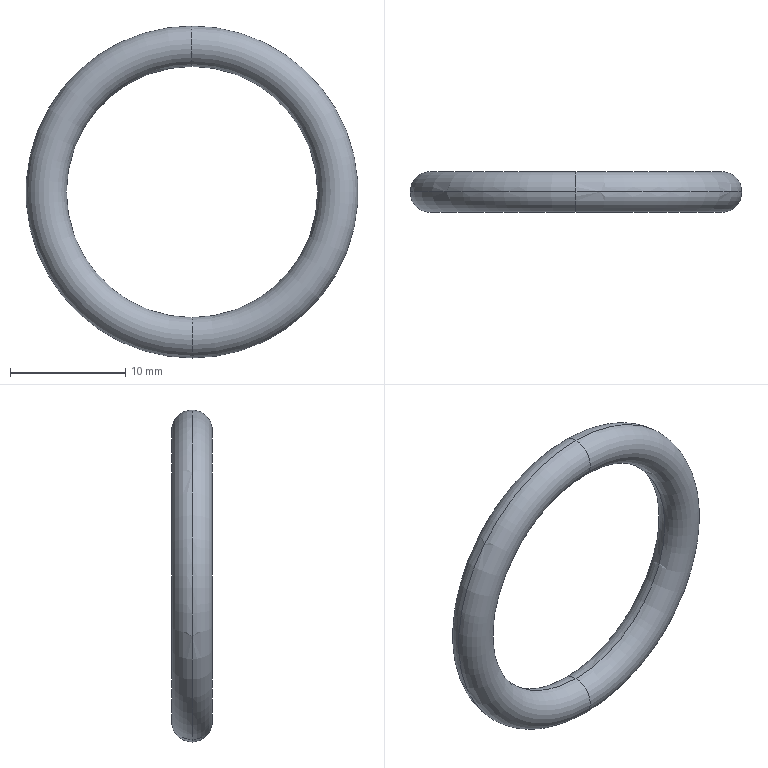Part | STEP file | TBS-1D91-0002_A0_O-RING_1 | 1 solid | 4 faces | box 28.75 x 3.5 x 28.75 mm | volume 763.198 mm3 | torus 4
STEP:
#1=CARTESIAN_POINT('',(0.,0.,0.));
#2=DIRECTION('',(0.,0.,1.));
#3=DIRECTION('',(1.,0.,0.));
#4=AXIS2_PLACEMENT_3D('',#1,#2,#3);
#5=CARTESIAN_POINT('',(0.,0.,-10.875));
#6=VERTEX_POINT('',#5);
#7=CARTESIAN_POINT('',(0.,0.,-14.375));
#8=VERTEX_POINT('',#7);
#9=CARTESIAN_POINT('',(0.,0.,-12.625));
#10=DIRECTION('',(1.,0.,0.));
#11=DIRECTION('',(0.,0.,1.));
#12=AXIS2_PLACEMENT_3D('',#9,#10,#11);
#13=CIRCLE('',#12,1.75);
#14=EDGE_CURVE('',#6,#8,#13,.T.);
#15=ORIENTED_EDGE('',*,*,#14,.F.);
#16=CARTESIAN_POINT('',(0.,0.,10.875));
#17=VERTEX_POINT('',#16);
#18=CARTESIAN_POINT('',(0.,0.,0.));
#19=DIRECTION('',(0.,1.,0.));
#20=DIRECTION('',(0.,0.,1.));
#21=AXIS2_PLACEMENT_3D('',#18,#19,#20);
#22=CIRCLE('',#21,10.875);
#23=EDGE_CURVE('',#17,#6,#22,.T.);
#24=ORIENTED_EDGE('',*,*,#23,.F.);
#25=CARTESIAN_POINT('',(0.,0.,14.375));
#26=VERTEX_POINT('',#25);
#27=CARTESIAN_POINT('',(0.,0.,12.625));
#28=DIRECTION('',(-1.,0.,0.));
#29=DIRECTION('',(0.,0.,-1.));
#30=AXIS2_PLACEMENT_3D('',#27,#28,#29);
#31=CIRCLE('',#30,1.75);
#32=EDGE_CURVE('',#17,#26,#31,.T.);
#33=ORIENTED_EDGE('',*,*,#32,.T.);
#34=CARTESIAN_POINT('',(0.,0.,0.));
#35=DIRECTION('',(0.,1.,0.));
#36=DIRECTION('',(0.,0.,1.));
#37=AXIS2_PLACEMENT_3D('',#34,#35,#36);
#38=CIRCLE('',#37,14.375);
#39=EDGE_CURVE('',#26,#8,#38,.T.);
#40=ORIENTED_EDGE('',*,*,#39,.T.);
#41=EDGE_LOOP('',(#15,#24,#33,#40));
#42=FACE_OUTER_BOUND('',#41,.F.);
#43=CARTESIAN_POINT('',(0.,0.,0.));
#44=DIRECTION('',(0.,-1.,0.));
#45=DIRECTION('',(0.,0.,-1.));
#46=AXIS2_PLACEMENT_3D('',#43,#44,#45);
#47=TOROIDAL_SURFACE('',#46,12.625,1.75);
#48=ADVANCED_FACE('',(#42),#47,.T.);
#49=ORIENTED_EDGE('',*,*,#32,.F.);
#50=CARTESIAN_POINT('',(0.,0.,0.));
#51=DIRECTION('',(0.,1.,0.));
#52=DIRECTION('',(0.,0.,-1.));
#53=AXIS2_PLACEMENT_3D('',#50,#51,#52);
#54=CIRCLE('',#53,10.875);
#55=EDGE_CURVE('',#6,#17,#54,.T.);
#56=ORIENTED_EDGE('',*,*,#55,.F.);
#57=ORIENTED_EDGE('',*,*,#14,.T.);
#58=CARTESIAN_POINT('',(0.,0.,0.));
#59=DIRECTION('',(0.,1.,0.));
#60=DIRECTION('',(0.,0.,-1.));
#61=AXIS2_PLACEMENT_3D('',#58,#59,#60);
#62=CIRCLE('',#61,14.375);
#63=EDGE_CURVE('',#8,#26,#62,.T.);
#64=ORIENTED_EDGE('',*,*,#63,.T.);
#65=EDGE_LOOP('',(#49,#56,#57,#64));
#66=FACE_OUTER_BOUND('',#65,.F.);
#67=CARTESIAN_POINT('',(0.,0.,0.));
#68=DIRECTION('',(0.,-1.,0.));
#69=DIRECTION('',(0.,0.,-1.));
#70=AXIS2_PLACEMENT_3D('',#67,#68,#69);
#71=TOROIDAL_SURFACE('',#70,12.625,1.75);
#72=ADVANCED_FACE('',(#66),#71,.T.);
#73=ORIENTED_EDGE('',*,*,#63,.F.);
#74=CARTESIAN_POINT('',(0.,0.,-12.625));
#75=DIRECTION('',(1.,0.,0.));
#76=DIRECTION('',(0.,0.,-1.));
#77=AXIS2_PLACEMENT_3D('',#74,#75,#76);
#78=CIRCLE('',#77,1.75);
#79=EDGE_CURVE('',#8,#6,#78,.T.);
#80=ORIENTED_EDGE('',*,*,#79,.T.);
#81=ORIENTED_EDGE('',*,*,#55,.T.);
#82=CARTESIAN_POINT('',(0.,0.,12.625));
#83=DIRECTION('',(-1.,0.,0.));
#84=DIRECTION('',(0.,0.,1.));
#85=AXIS2_PLACEMENT_3D('',#82,#83,#84);
#86=CIRCLE('',#85,1.75);
#87=EDGE_CURVE('',#26,#17,#86,.T.);
#88=ORIENTED_EDGE('',*,*,#87,.F.);
#89=EDGE_LOOP('',(#73,#80,#81,#88));
#90=FACE_OUTER_BOUND('',#89,.F.);
#91=CARTESIAN_POINT('',(0.,0.,0.));
#92=DIRECTION('',(0.,-1.,0.));
#93=DIRECTION('',(0.,0.,-1.));
#94=AXIS2_PLACEMENT_3D('',#91,#92,#93);
#95=TOROIDAL_SURFACE('',#94,12.625,1.75);
#96=ADVANCED_FACE('',(#90),#95,.T.);
#97=ORIENTED_EDGE('',*,*,#39,.F.);
#98=ORIENTED_EDGE('',*,*,#87,.T.);
#99=ORIENTED_EDGE('',*,*,#23,.T.);
#100=ORIENTED_EDGE('',*,*,#79,.F.);
#101=EDGE_LOOP('',(#97,#98,#99,#100));
#102=FACE_OUTER_BOUND('',#101,.F.);
#103=CARTESIAN_POINT('',(0.,0.,0.));
#104=DIRECTION('',(0.,-1.,0.));
#105=DIRECTION('',(0.,0.,-1.));
#106=AXIS2_PLACEMENT_3D('',#103,#104,#105);
#107=TOROIDAL_SURFACE('',#106,12.625,1.75);
#108=ADVANCED_FACE('',(#102),#107,.T.);
#109=CLOSED_SHELL('',(#48,#72,#96,#108));
#110=MANIFOLD_SOLID_BREP('',#109);
#111=(LENGTH_UNIT()NAMED_UNIT(*)SI_UNIT(.MILLI.,.METRE.));
#112=UNCERTAINTY_MEASURE_WITH_UNIT(LENGTH_MEASURE(0.004081),#111,'','');
#113=(NAMED_UNIT(*)PLANE_ANGLE_UNIT()SI_UNIT($,.RADIAN.));
#114=PLANE_ANGLE_MEASURE_WITH_UNIT(PLANE_ANGLE_MEASURE(0.01745),#113);
#115=(CONVERSION_BASED_UNIT('DEGREE',#114)NAMED_UNIT(*)PLANE_ANGLE_UNIT());
#116=(NAMED_UNIT(*)SI_UNIT($,.STERADIAN.)SOLID_ANGLE_UNIT());
#117=(GEOMETRIC_REPRESENTATION_CONTEXT(3)GLOBAL_UNCERTAINTY_ASSIGNED_CONTEXT((#112))GLOBAL_UNIT_ASSIGNED_CONTEXT((#111,#115,#116))REPRESENTATION_CONTEXT('',''));
#118=ADVANCED_BREP_SHAPE_REPRESENTATION('',(#4,#110),#117);